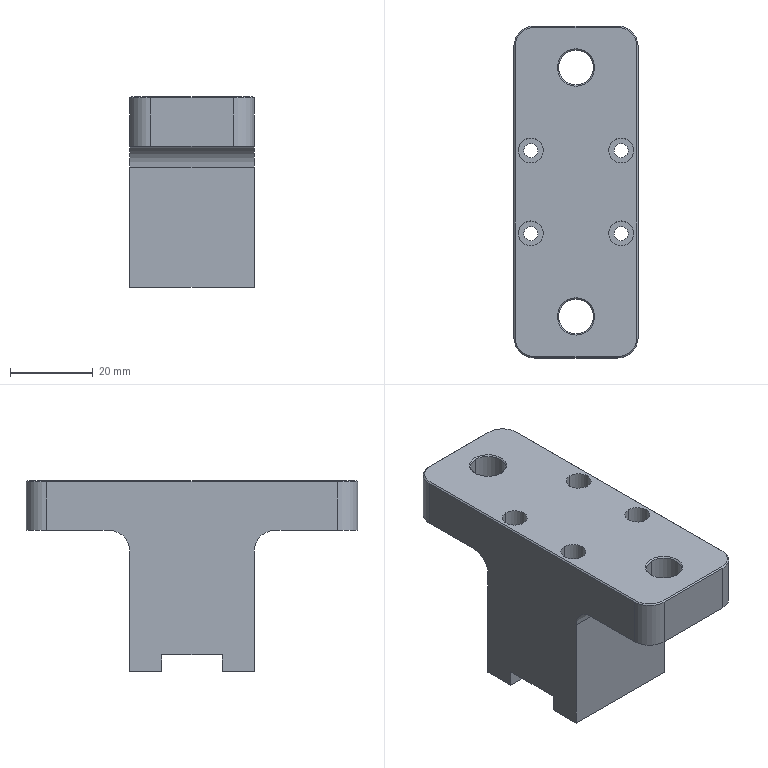NC program | NX | posted with a generic post | part box 30 x 80 x 46 mm
Lines 19 to 1040 of 3641:
(ZLEVEL_PROFILE , TOOL : D10)
N36 T15 M6
N38 G54
N40 G17 G0 G90 X-38.948 Y-19.275 S9500 M3
N42 G43 Z30. H15
N44 Z1.5
N46 G94 G1 X-39.694 Y-18.977 Z1.458 F1000.
N48 X-41.403 Y-17.85 Z1.351
N50 X-42.85 Y-16.403 Z1.243
N52 X-43.977 Y-14.694 Z1.136
N54 X-44.737 Y-12.793 Z1.029
N56 X-45.1 Y-10.779 Z0.922
N58 Y10.779 Z-0.208
N60 X-44.737 Y12.793 Z-0.316
N62 X-43.977 Y14.694 Z-0.423
N64 X-42.85 Y16.403 Z-0.53
N66 X-41.403 Y17.85 Z-0.637
N68 X-39.694 Y18.977 Z-0.745
N70 X-37.793 Y19.737 Z-0.852
N72 X-35.779 Y20.1 Z-0.959
N74 X-35. Z-1.
N76 X35. F3000.
N78 G2 X45.1 Y10. R10.1
N80 G1 Y-10.
N82 G2 X35. Y-20.1 R10.1
N84 G1 X-35.
N86 G2 X-45.1 Y-10. R10.1
N88 G1 Y10.
N90 G2 X-35. Y20.1 R10.1
N92 G1 X22.29 Z-2.
N94 X35.
N96 G2 X45.1 Y10. R10.1
N98 G1 Y-10.
N100 G2 X35. Y-20.1 R10.1
N102 G1 X-35.
N104 G2 X-45.1 Y-10. R10.1
N106 G1 Y10.
N108 G2 X-35. Y20.1 R10.1
N110 G1 X22.29 Z-3.
N112 X35.
N114 G2 X45.1 Y10. R10.1
N116 G1 Y-10.
N118 G2 X35. Y-20.1 R10.1
N120 G1 X-35.
N122 G2 X-45.1 Y-10. R10.1
N124 G1 Y10.
N126 G2 X-35. Y20.1 R10.1
N128 G1 X22.29 Z-4.
N130 X35.
N132 G2 X45.1 Y10. R10.1
N134 G1 Y-10.
N136 G2 X35. Y-20.1 R10.1
N138 G1 X-35.
N140 G2 X-45.1 Y-10. R10.1
N142 G1 Y10.
N144 G2 X-35. Y20.1 R10.1
N146 G1 X22.29 Z-5.
N148 X35.
N150 G2 X45.1 Y10. R10.1
N152 G1 Y-10.
N154 G2 X35. Y-20.1 R10.1
N156 G1 X-35.
N158 G2 X-45.1 Y-10. R10.1
N160 G1 Y10.
N162 G2 X-35. Y20.1 R10.1
N164 G1 X22.29 Z-6.
N166 X35.
N168 G2 X45.1 Y10. R10.1
N170 G1 Y-10.
N172 G2 X35. Y-20.1 R10.1
N174 G1 X-35.
N176 G2 X-45.1 Y-10. R10.1
N178 G1 Y10.
N180 G2 X-35. Y20.1 R10.1
N182 G1 X22.29 Z-7.
N184 X35.
N186 G2 X45.1 Y10. R10.1
N188 G1 Y-10.
N190 G2 X35. Y-20.1 R10.1
N192 G1 X-35.
N194 G2 X-45.1 Y-10. R10.1
N196 G1 Y10.
N198 G2 X-35. Y20.1 R10.1
N200 G1 X22.29 Z-8.
N202 X35.
N204 G2 X45.1 Y10. R10.1
N206 G1 Y-10.
N208 G2 X35. Y-20.1 R10.1
N210 G1 X-35.
N212 G2 X-45.1 Y-10. R10.1
N214 G1 Y10.
N216 G2 X-35. Y20.1 R10.1
N218 G1 X22.29 Z-9.
N220 X35.
N222 G2 X45.1 Y10. R10.1
N224 G1 Y-10.
N226 G2 X35. Y-20.1 R10.1
N228 G1 X-35.
N230 G2 X-45.1 Y-10. R10.1
N232 G1 Y10.
N234 G2 X-35. Y20.1 R10.1
N236 G1 X22.29 Z-10.
N238 X35.
N240 G2 X45.1 Y10. R10.1
N242 G1 Y-10.
N244 G2 X35. Y-20.1 R10.1
N246 G1 X-35.
N248 G2 X-45.1 Y-10. R10.1
N250 G1 Y10.
N252 G2 X-35. Y20.1 R10.1
N254 G1 X22.29 Z-11.
N256 X35.
N258 G2 X45.1 Y10. R10.1
N260 G1 Y-10.
N262 G2 X35. Y-20.1 R10.1
N264 G1 X-35.
N266 G2 X-45.1 Y-10. R10.1
N268 G1 Y10.
N270 G2 X-35. Y20.1 R10.1
N272 G1 X22.29 Z-12.
N274 X35.
N276 G2 X45.1 Y10. R10.1
N278 G1 Y-10.
N280 G2 X35. Y-20.1 R10.1
N282 G1 X-35.
N284 G2 X-45.1 Y-10. R10.1
N286 G1 Y10.
N288 G2 X-35. Y20.1 R10.1
N290 G1 X22.29 Z-13.
N292 X35.
N294 G2 X45.1 Y10. R10.1
N296 G1 Y-10.
N298 G2 X35. Y-20.1 R10.1
N300 G1 X-35.
N302 G2 X-45.1 Y-10. R10.1
N304 G1 Y10.
N306 G2 X-35. Y20.1 R10.1
N308 G1 X22.29 Z-14.
N310 X35.
N312 G2 X45.1 Y10. R10.1
N314 G1 Y-10.
N316 G2 X35. Y-20.1 R10.1
N318 G1 X-35.
N320 G2 X-45.1 Y-10. R10.1
N322 G1 Y10.
N324 G2 X-35. Y20.1 R10.1
N326 G1 X22.29 Z-15.
N328 X35.
N330 G2 X45.1 Y10. R10.1
N332 G1 Y-10.
N334 G2 X35. Y-20.1 R10.1
N336 G1 X-35.
N338 G2 X-45.1 Y-10. R10.1
N340 G1 Y10.
N342 G2 X-35. Y20.1 R10.1
N344 G1 X22.29 Z-16.
N346 X35.
N348 G2 X45.1 Y10. R10.1
N350 G1 Y-10.
N352 G2 X35. Y-20.1 R10.1
N354 G1 X-35.
N356 G2 X-45.1 Y-10. R10.1
N358 G1 Y10.
N360 G2 X-35. Y20.1 R10.1
N362 G1 X22.29 Z-17.
N364 X35.
N366 G2 X45.1 Y10. R10.1
N368 G1 Y-10.
N370 G2 X35. Y-20.1 R10.1
N372 G1 X-35.
N374 G2 X-45.1 Y-10. R10.1
N376 G1 Y10.
N378 G2 X-35. Y20.1 R10.1
N380 G1 X22.29 Z-18.
N382 X35.
N384 G2 X45.1 Y10. R10.1
N386 G1 Y-10.
N388 G2 X35. Y-20.1 R10.1
N390 G1 X-35.
N392 G2 X-45.1 Y-10. R10.1
N394 G1 Y10.
N396 G2 X-35. Y20.1 R10.1
N398 G1 X22.29 Z-19.
N400 X35.
N402 G2 X45.1 Y10. R10.1
N404 G1 Y-10.
N406 G2 X35. Y-20.1 R10.1
N408 G1 X-35.
N410 G2 X-45.1 Y-10. R10.1
N412 G1 Y10.
N414 G2 X-35. Y20.1 R10.1
N416 G1 X22.29 Z-20.
N418 X35.
N420 G2 X45.1 Y10. R10.1
N422 G1 Y-10.
N424 G2 X35. Y-20.1 R10.1
N426 G1 X-35.
N428 G2 X-45.1 Y-10. R10.1
N430 G1 Y10.
N432 G2 X-35. Y20.1 R10.1
N434 G1 X22.29 Z-21.
N436 X35.
N438 G2 X45.1 Y10. R10.1
N440 G1 Y-10.
N442 G2 X35. Y-20.1 R10.1
N444 G1 X-35.
N446 G2 X-45.1 Y-10. R10.1
N448 G1 Y10.
N450 G2 X-35. Y20.1 R10.1
N452 G1 X22.29 Z-22.
N454 X35.
N456 G2 X45.1 Y10. R10.1
N458 G1 Y-10.
N460 G2 X35. Y-20.1 R10.1
N462 G1 X-35.
N464 G2 X-45.1 Y-10. R10.1
N466 G1 Y10.
N468 G2 X-35. Y20.1 R10.1
N470 G1 X22.29 Z-23.
N472 X35.
N474 G2 X45.1 Y10. R10.1
N476 G1 Y-10.
N478 G2 X35. Y-20.1 R10.1
N480 G1 X-35.
N482 G2 X-45.1 Y-10. R10.1
N484 G1 Y10.
N486 G2 X-35. Y20.1 R10.1
N488 G1 X22.29 Z-24.
N490 X35.
N492 G2 X45.1 Y10. R10.1
N494 G1 Y-10.
N496 G2 X35. Y-20.1 R10.1
N498 G1 X-35.
N500 G2 X-45.1 Y-10. R10.1
N502 G1 Y10.
N504 G2 X-35. Y20.1 R10.1
N506 G1 X22.29 Z-25.
N508 X35.
N510 G2 X45.1 Y10. R10.1
N512 G1 Y-10.
N514 G2 X35. Y-20.1 R10.1
N516 G1 X-35.
N518 G2 X-45.1 Y-10. R10.1
N520 G1 Y10.
N522 G2 X-35. Y20.1 R10.1
N524 G1 X22.29 Z-26.
N526 X35.
N528 G2 X45.1 Y10. R10.1
N530 G1 Y-10.
N532 G2 X35. Y-20.1 R10.1
N534 G1 X-35.
N536 G2 X-45.1 Y-10. R10.1
N538 G1 Y10.
N540 G2 X-35. Y20.1 R10.1
N542 G1 X22.29 Z-27.
N544 X35.
N546 G2 X45.1 Y10. R10.1
N548 G1 Y-10.
N550 G2 X35. Y-20.1 R10.1
N552 G1 X-35.
N554 G2 X-45.1 Y-10. R10.1
N556 G1 Y10.
N558 G2 X-35. Y20.1 R10.1
N560 G1 X22.29 Z-28.
N562 X35.
N564 G2 X45.1 Y10. R10.1
N566 G1 Y-10.
N568 G2 X35. Y-20.1 R10.1
N570 G1 X-35.
N572 G2 X-45.1 Y-10. R10.1
N574 G1 Y10.
N576 G2 X-35. Y20.1 R10.1
N578 G1 X22.29 Z-29.
N580 X35.
N582 G2 X45.1 Y10. R10.1
N584 G1 Y-10.
N586 G2 X35. Y-20.1 R10.1
N588 G1 X-35.
N590 G2 X-45.1 Y-10. R10.1
N592 G1 Y10.
N594 G2 X-35. Y20.1 R10.1
N596 G1 X22.29 Z-30.
N598 X35.
N600 G2 X45.1 Y10. R10.1
N602 G1 Y-10.
N604 G2 X35. Y-20.1 R10.1
N606 G1 X-35.
N608 G2 X-45.1 Y-10. R10.1
N610 G1 Y10.
N612 G2 X-35. Y20.1 R10.1
N614 G1 X22.29 Z-31.
N616 X35.
N618 G2 X45.1 Y10. R10.1
N620 G1 Y-10.
N622 G2 X35. Y-20.1 R10.1
N624 G1 X-35.
N626 G2 X-45.1 Y-10. R10.1
N628 G1 Y10.
N630 G2 X-35. Y20.1 R10.1
N632 G1 X22.29 Z-32.
N634 X35.
N636 G2 X45.1 Y10. R10.1
N638 G1 Y-10.
N640 G2 X35. Y-20.1 R10.1
N642 G1 X-35.
N644 G2 X-45.1 Y-10. R10.1
N646 G1 Y10.
N648 G2 X-35. Y20.1 R10.1
N650 G1 X22.29 Z-33.
N652 X35.
N654 G2 X45.1 Y10. R10.1
N656 G1 Y-10.
N658 G2 X35. Y-20.1 R10.1
N660 G1 X-35.
N662 G2 X-45.1 Y-10. R10.1
N664 G1 Y10.
N666 G2 X-35. Y20.1 R10.1
N668 G1 X22.29 Z-34.
N670 X35.
N672 G2 X45.1 Y10. R10.1
N674 G1 Y-10.
N676 G2 X35. Y-20.1 R10.1
N678 G1 X-35.
N680 G2 X-45.1 Y-10. R10.1
N682 G1 Y10.
N684 G2 X-35. Y20.1 R10.1
N686 G1 X22.29 Z-35.
N688 X35.
N690 G2 X45.1 Y10. R10.1
N692 G1 Y-10.
N694 G2 X35. Y-20.1 R10.1
N696 G1 X-35.
N698 G2 X-45.1 Y-10. R10.1
N700 G1 Y10.
N702 G2 X-35. Y20.1 R10.1
N704 G1 X22.29 Z-36.
N706 X35.
N708 G2 X45.1 Y10. R10.1
N710 G1 Y-10.
N712 G2 X35. Y-20.1 R10.1
N714 G1 X-35.
N716 G2 X-45.1 Y-10. R10.1
N718 G1 Y10.
N720 G2 X-35. Y20.1 R10.1
N722 G1 X22.29 Z-37.
N724 X35.
N726 G2 X45.1 Y10. R10.1
N728 G1 Y-10.
N730 G2 X35. Y-20.1 R10.1
N732 G1 X-35.
N734 G2 X-45.1 Y-10. R10.1
N736 G1 Y10.
N738 G2 X-35. Y20.1 R10.1
N740 G1 X22.29 Z-38.
N742 X35.
N744 G2 X45.1 Y10. R10.1
N746 G1 Y-10.
N748 G2 X35. Y-20.1 R10.1
N750 G1 X-35.
N752 G2 X-45.1 Y-10. R10.1
N754 G1 Y10.
N756 G2 X-35. Y20.1 R10.1
N758 G1 X22.29 Z-39.
N760 X35.
N762 G2 X45.1 Y10. R10.1
N764 G1 Y-10.
N766 G2 X35. Y-20.1 R10.1
N768 G1 X-35.
N770 G2 X-45.1 Y-10. R10.1
N772 G1 Y10.
N774 G2 X-35. Y20.1 R10.1
N776 G1 X22.29 Z-40.
N778 X35.
N780 G2 X45.1 Y10. R10.1
N782 G1 Y-10.
N784 G2 X35. Y-20.1 R10.1
N786 G1 X-35.
N788 G2 X-45.1 Y-10. R10.1
N790 G1 Y10.
N792 G2 X-35. Y20.1 R10.1
N794 G1 X22.29 Z-41.
N796 X35.
N798 G2 X45.1 Y10. R10.1
N800 G1 Y-10.
N802 G2 X35. Y-20.1 R10.1
N804 G1 X-35.
N806 G2 X-45.1 Y-10. R10.1
N808 G1 Y10.
N810 G2 X-35. Y20.1 R10.1
N812 G1 X22.29 Z-42.
N814 X35.
N816 G2 X45.1 Y10. R10.1
N818 G1 Y-10.
N820 G2 X35. Y-20.1 R10.1
N822 G1 X-35.
N824 G2 X-45.1 Y-10. R10.1
N826 G1 Y10.
N828 G2 X-35. Y20.1 R10.1
N830 G1 X22.29 Z-43.
N832 X35.
N834 G2 X45.1 Y10. R10.1
N836 G1 Y-10.
N838 G2 X35. Y-20.1 R10.1
N840 G1 X-35.
N842 G2 X-45.1 Y-10. R10.1
N844 G1 Y10.
N846 G2 X-35. Y20.1 R10.1
N848 G1 X22.29 Z-44.
N850 X35.
N852 G2 X45.1 Y10. R10.1
N854 G1 Y-10.
N856 G2 X35. Y-20.1 R10.1
N858 G1 X-35.
N860 G2 X-45.1 Y-10. R10.1
N862 G1 Y10.
N864 G2 X-35. Y20.1 R10.1
N866 G1 X22.29 Z-45.
N868 X35.
N870 G2 X45.1 Y10. R10.1
N872 G1 Y-10.
N874 G2 X35. Y-20.1 R10.1
N876 G1 X-35.
N878 G2 X-45.1 Y-10. R10.1
N880 G1 Y10.
N882 G2 X-35. Y20.1 R10.1
N884 G1 X22.29 Z-46.
N886 X35.
N888 G2 X45.1 Y10. R10.1
N890 G1 Y-10.
N892 G2 X35. Y-20.1 R10.1
N894 G1 X-35.
N896 G2 X-45.1 Y-10. R10.1
N898 G1 Y10.
N900 G2 X-35. Y20.1 R10.1
N902 G1 X22.29
N904 Z-44.5
N906 G0 Z30.
(ZLEVEL_PROFILE_COPY_COPY_COPY , TOOL : D10)
N908 X40.999 Y21.367
N910 Z-0.997
N912 G1 X39.499 Y20.501 F1000.
N914 G3 X38.999 Y19.635 R1.
N916 G1 X39. Y14.376 F3000.
N918 Y-15.
N920 X38.999 Y-19.635
N922 G3 X39.499 Y-20.501 R1.
N924 G1 X40.999 Y-21.367
N926 G0 X40.998 Y-21.395 Z-1.994
N928 G1 X39.499 Y-20.529 F1000.
N930 G2 X38.999 Y-19.663 R1.
N932 G1 X39. Y-15. F3000.
N934 Y14.376
N936 X38.999 Y19.663
N938 G2 X39.499 Y20.529 R1.
N940 G1 X40.998 Y21.395
N942 G0 X40.996 Y21.422 Z-2.991
N944 G1 X39.499 Y20.558 F1000.
N946 G3 X38.999 Y19.692 R1.
N948 G1 X39. Y14.376 F3000.
N950 Y-15.
N952 X38.999 Y-19.692
N954 G3 X39.499 Y-20.558 R1.
N956 G1 X40.996 Y-21.422
N958 G0 X40.994 Y-21.449 Z-3.988
N960 G1 X39.499 Y-20.586 F1000.
N962 G2 X38.999 Y-19.72 R1.
N964 G1 X39. Y-15. F3000.
N966 Y14.376
N968 X38.999 Y19.72
N970 G2 X39.499 Y20.586 R1.
N972 G1 X40.994 Y21.449
N974 G0 X40.992 Y21.477 Z-4.985
N976 G1 X39.499 Y20.615 F1000.
N978 G3 X38.999 Y19.749 R1.
N980 G1 X39. Y14.376 F3000.
N982 Y-15.
N984 X38.999 Y-19.748
N986 G3 X39.499 Y-20.615 R1.
N988 G1 X40.992 Y-21.477
N990 G0 X40.99 Y-21.504 Z-5.982
N992 G1 X39.499 Y-20.643 F1000.
N994 G2 X38.999 Y-19.777 R1.
N996 G1 X39. Y-15. F3000.
N998 Y14.376
N1000 X38.999 Y19.777
N1002 G2 X39.499 Y20.643 R1.
N1004 G1 X40.99 Y21.504
N1006 G0 X40.988 Y21.548 Z-6.979
N1008 G1 X39.494 Y20.674 F1000.
N1010 G3 X38.999 Y19.805 R1.
N1012 G1 X39.001 Y19.45 F3000.
N1014 X39. Y14.376
N1016 Y-15.
N1018 X39.001 Y-19.45
N1020 X38.999 Y-19.805
N1022 G3 X39.494 Y-20.674 R1.
N1024 G1 X40.988 Y-21.548
N1026 G0 X40.986 Y-21.575 Z-7.976
N1028 G1 X39.494 Y-20.702 F1000.
N1030 G2 X38.999 Y-19.834 R1.
N1032 G1 X39.002 Y-19.45 F3000.
N1034 X39. Y-15.
N1036 Y14.376
N1038 X39.002 Y19.45
N1040 X38.999 Y19.834
N1042 G2 X39.494 Y20.703 R1.
N1044 G1 X40.986 Y21.575
N1046 G0 X40.984 Y21.603 Z-8.974
N1048 G1 X39.494 Y20.731 F1000.
N1050 G3 X38.999 Y19.862 R1.
N1052 G1 X39.002 Y19.45 F3000.
N1054 X39. Y14.376
N1056 Y-15.
N1058 X39.002 Y-19.45
N1060 X38.999 Y-19.862
N1062 G3 X39.494 Y-20.731 R1.
N1064 G1 X40.984 Y-21.603
N1066 G0 X40.982 Y-21.63 Z-9.971
N1068 G1 X39.494 Y-20.759 F1000.
N1070 G2 X38.999 Y-19.89 R1.
N1072 G1 X39.002 Y-19.45 F3000.
N1074 X39. Y-15.
N1076 Y14.376
N1078 X39.002 Y19.45
N1080 X38.999 Y19.89
N1082 G2 X39.494 Y20.759 R1.
N1084 G1 X40.982 Y21.63
N1086 G0 X40.98 Y21.658 Z-10.968
N1088 G1 X39.494 Y20.788 F1000.
N1090 G3 X38.999 Y19.919 R1.
N1092 G1 X39.002 Y19.45 F3000.
N1094 X39. Y14.376
N1096 Y-15.
N1098 X39.002 Y-19.45
N1100 X38.999 Y-19.919
N1102 G3 X39.494 Y-20.788 R1.
N1104 G1 X40.98 Y-21.658
N1106 G0 X40.978 Y-21.685 Z-11.965
N1108 G1 X39.494 Y-20.816 F1000.
N1110 G2 X38.999 Y-19.947 R1.
N1112 G1 X39.002 Y-19.45 F3000.
N1114 X39. Y-15.
N1116 Y14.376
N1118 X39.002 Y19.45
N1120 X38.999 Y19.947
N1122 G2 X39.494 Y20.816 R1.
N1124 G1 X40.978 Y21.685
N1126 G0 X40.976 Y21.713 Z-12.962
N1128 G1 X39.494 Y20.844 F1000.
N1130 G3 X38.999 Y19.975 R1.
N1132 G1 X39.002 Y19.45 F3000.
N1134 X39. Y14.376
N1136 Y-15.
N1138 X39.002 Y-19.45
N1140 X38.999 Y-19.975
N1142 G3 X39.494 Y-20.844 R1.
N1144 G1 X40.976 Y-21.713
N1146 G0 X40.974 Y-21.74 Z-13.959
N1148 G1 X39.493 Y-20.873 F1000.
N1150 G2 X38.999 Y-20.004 R1.
N1152 G1 X39.002 Y-19.45 F3000.
N1154 X39. Y-15.
N1156 Y14.376
N1158 X39.002 Y19.45
N1160 X38.999 Y20.004
N1162 G2 X39.493 Y20.873 R1.
N1164 G1 X40.974 Y21.74
N1166 G0 X40.972 Y21.768 Z-14.956
N1168 G1 X39.493 Y20.901 F1000.
N1170 G3 X38.999 Y20.032 R1.
N1172 G1 X39.003 Y19.45 F3000.
N1174 X39. Y14.376
N1176 Y-15.
N1178 X39.003 Y-19.45
N1180 X38.999 Y-20.032
N1182 G3 X39.493 Y-20.901 R1.
N1184 G1 X40.972 Y-21.768
N1186 G0 X40.97 Y-21.795 Z-15.953
N1188 G1 X39.493 Y-20.93 F1000.
N1190 G2 X38.999 Y-20.06 R1.
N1192 G1 X39.003 Y-19.45 F3000.
N1194 X39. Y-15.
N1196 Y14.376
N1198 X39.003 Y19.45
N1200 X38.999 Y20.06
N1202 G2 X39.493 Y20.93 R1.
N1204 G1 X40.97 Y21.795
N1206 G0 X40.968 Y21.823 Z-16.95
N1208 G1 X39.493 Y20.958 F1000.
N1210 G3 X38.999 Y20.089 R1.
N1212 G1 X39.003 Y19.45 F3000.
N1214 X39. Y14.376
N1216 Y-15.
N1218 X39.003 Y-19.45
N1220 X38.999 Y-20.089
N1222 G3 X39.493 Y-20.958 R1.
N1224 G1 X40.968 Y-21.823
N1226 G0 X40.967 Y-21.85 Z-17.947
N1228 G1 X39.493 Y-20.986 F1000.
N1230 G2 X38.999 Y-20.117 R1.
N1232 G1 X39.003 Y-19.45 F3000.
N1234 X39. Y-15.
N1236 Y14.376
N1238 X39.003 Y19.45
N1240 X38.999 Y20.117
N1242 G2 X39.493 Y20.986 R1.
N1244 G1 X40.967 Y21.85
N1246 G0 X40.965 Y21.878 Z-18.944
N1248 G1 X39.493 Y21.015 F1000.
N1250 G3 X38.998 Y20.145 R1.
N1252 G1 X39.003 Y19.45 F3000.
N1254 X39. Y14.376
N1256 Y-15.
N1258 X39.003 Y-19.45
N1260 X38.998 Y-20.145
N1262 G3 X39.493 Y-21.015 R1.
N1264 G1 X40.965 Y-21.878
N1266 G0 X40.963 Y-21.905 Z-19.941
N1268 G1 X39.493 Y-21.043 F1000.
N1270 G2 X38.998 Y-20.174 R1.
N1272 G1 X39.003 Y-19.45 F3000.
N1274 X39. Y-15.
N1276 Y14.376
N1278 Y15.021
N1280 X39.003 Y19.45
N1282 X38.998 Y20.174
N1284 G2 X39.493 Y21.043 R1.
N1286 G1 X40.963 Y21.905
N1288 G0 X40.961 Y21.933 Z-20.938
N1290 G1 X39.492 Y21.071 F1000.
N1292 G3 X38.998 Y20.202 R1.
N1294 G1 X39.003 Y19.45 F3000.
N1296 X39. Y15.021
N1298 Y14.376
N1300 Y-15.
N1302 X39.003 Y-19.45
N1304 X38.998 Y-20.202
N1306 G3 X39.492 Y-21.071 R1.
N1308 G1 X40.961 Y-21.933
N1310 G0 X40.959 Y-21.96 Z-21.935
N1312 G1 X39.492 Y-21.1 F1000.
N1314 G2 X38.998 Y-20.23 R1.
N1316 G1 X39.004 Y-19.45 F3000.
N1318 X39. Y-15.
N1320 Y14.376
N1322 Y15.021
N1324 X39.004 Y19.45
N1326 X38.998 Y20.23
N1328 G2 X39.492 Y21.1 R1.
N1330 G1 X40.959 Y21.96
N1332 G0 X40.957 Y21.988 Z-22.932
N1334 G1 X39.492 Y21.128 F1000.
N1336 G3 X38.998 Y20.259 R1.
N1338 G1 X39.004 Y19.45 F3000.
N1340 X39. Y15.021
N1342 Y14.376
N1344 Y-15.
N1346 X39.004 Y-19.45
N1348 X38.998 Y-20.259
N1350 G3 X39.492 Y-21.128 R1.
N1352 G1 X40.957 Y-21.987
N1354 G0 X40.955 Y-22.015 Z-23.929
N1356 G1 X39.492 Y-21.156 F1000.
N1358 G2 X38.998 Y-20.287 R1.
N1360 G1 X39.004 Y-19.45 F3000.
N1362 X39. Y-15.
N1364 Y14.376
N1366 Y15.021
N1368 X39.004 Y19.45
N1370 X38.998 Y20.287
N1372 G2 X39.492 Y21.157 R1.
N1374 G1 X40.955 Y22.015
N1376 G0 X40.954 Y22.023 Z-24.926
N1378 G1 X39.498 Y21.182 F1000.
N1380 G3 X38.998 Y20.315 R1.
N1382 G1 X39. Y14.376 F3000.
N1384 Y-15.
N1386 X39.004 Y-19.45
N1388 X38.998 Y-20.315
N1390 G3 X39.492 Y-21.185 R1.
N1392 G1 X40.953 Y-22.042
N1394 G0 X40.951 Y-22.07 Z-25.924
N1396 G1 X39.491 Y-21.213 F1000.
N1398 G2 X38.998 Y-20.343 R1.
N1400 G1 X39.004 Y-19.45 F3000.
N1402 X39. Y-15.
N1404 Y14.376
N1406 X38.998 Y20.344
N1408 G2 X39.497 Y21.21 R1.
N1410 G1 X40.952 Y22.051
N1412 G0 X40.95 Y22.078 Z-26.921
N1414 G1 X39.497 Y21.238 F1000.
N1416 G3 X38.998 Y20.372 R1.
N1418 G1 X39. Y14.376 F3000.
N1420 Y-15.
N1422 X39.004 Y-19.45
N1424 X38.998 Y-20.372
N1426 G3 X39.491 Y-21.241 R1.
N1428 G1 X40.949 Y-22.097
N1430 G0 X40.947 Y-22.125 Z-27.918
N1432 G1 X39.491 Y-21.27 F1000.
N1434 G2 X38.997 Y-20.4 R1.
N1436 G1 X39.004 Y-19.45 F3000.
N1438 X39. Y-15.
N1440 Y14.376
N1442 X38.997 Y20.4
N1444 G2 X39.497 Y21.266 R1.
N1446 G1 X40.948 Y22.105
N1448 G0 X40.946 Y22.132 Z-28.915
N1450 G1 X39.497 Y21.295 F1000.
N1452 G3 X38.997 Y20.429 R1.
N1454 G1 X38.999 Y14.793 F3000.
N1456 X39. Y14.376
N1458 Y-15.
N1460 X39.005 Y-19.45
N1462 X38.997 Y-20.428
N1464 G3 X39.491 Y-21.298 R1.
N1466 G1 X40.945 Y-22.152
N1468 G0 X41.131 Y-22.176 Z-29.912
N1470 G1 X39.68 Y-21.33 F1000.
N1472 G2 X39.184 Y-20.462 R1.
N1474 G3 X39.084 Y-14.689 R134.164 F3000.
N1476 G1 Y14.793
N1478 G3 X39.165 Y20.459 R86.418
N1480 G2 X39.649 Y21.334 R1.
N1482 G1 X41.109 Y22.214
N1484 G0 X41.473 Y22.246 Z-30.909
N1486 G1 X39.998 Y21.363 F1000.
N1488 G3 X39.512 Y20.49 R1.
N1490 G2 X39.435 Y14.974 R93.208 F3000.
N1492 G1 X39.411 Y14.61
N1494 X39.379 Y14.552
N1496 Y-14.534
N1498 X39.405 Y-14.614
N1500 X39.49 Y-16.067
N1502 X39.499 Y-16.7
N1504 X39.512 Y-20.489
N1506 G3 X40.015 Y-21.354 R1.
N1508 G1 X41.463 Y-22.183
N1510 G0 X42.044 Y-22.251 Z-31.906
N1512 G1 X40.585 Y-21.374 F1000.
N1514 G2 X40.101 Y-20.499 R1.
N1516 G3 X39.975 Y-14.376 R79.288 F3000.
N1518 G1 X39.931 Y-14.264
N1520 Y14.264
N1522 X39.975 Y14.376
N1524 G3 X40.101 Y20.499 R79.291
N1526 G2 X40.585 Y21.374 R1.
N1528 G1 X42.044 Y22.252
N1530 G0 X43.052 Y22.297 Z-32.903
N1532 G1 X41.589 Y21.382 F1000.
N1534 G3 X41.12 Y20.5 R1.
N1536 G2 X40.875 Y13.953 R45.316 F3000.
N1538 G1 Y-13.953
N1540 G2 X41.12 Y-20.499 R45.314
N1542 G3 X41.589 Y-21.382 R1.
N1544 G1 X43.059 Y-22.301
N1546 G0 X45.387 Y-21.571 Z-33.9
N1548 G1 X43.95 Y-20.813 F1000.
N1550 G2 X43.417 Y-19.966 R1.
N1552 G1 X43.205 Y-14.376 F3000.
N1554 X43.005 Y-13.22
N1556 Y13.869
N1558 X43.136 Y14.376
N1560 X43.468 Y19.894
N1562 G2 X44.019 Y20.729 R1.
N1564 G1 X45.359 Y21.399
N1566 G0 Z30.
N1568 X-40.999 Y-21.367
N1570 Z-0.997
N1572 G1 X-39.499 Y-20.501 F1000.
N1574 G3 X-38.999 Y-19.635 R1.
N1576 G1 X-39. Y-14.961 F3000.
N1578 Y14.376
N1580 X-38.999 Y19.635
N1582 G3 X-39.499 Y20.501 R1.
N1584 G1 X-40.999 Y21.367
N1586 G0 X-40.998 Y21.395 Z-1.994
N1588 G1 X-39.499 Y20.529 F1000.
N1590 G2 X-38.999 Y19.663 R1.
N1592 G1 X-39. Y14.376 F3000.
N1594 Y-14.961
N1596 X-38.999 Y-19.663
N1598 G2 X-39.499 Y-20.529 R1.
N1600 G1 X-40.998 Y-21.395
N1602 G0 X-40.996 Y-21.422 Z-2.991
N1604 G1 X-39.499 Y-20.558 F1000.
N1606 G3 X-38.999 Y-19.692 R1.
N1608 G1 X-39. Y-14.961 F3000.
N1610 Y14.376
N1612 X-38.999 Y19.692
N1614 G3 X-39.499 Y20.558 R1.
N1616 G1 X-40.996 Y21.422
N1618 G0 X-40.994 Y21.449 Z-3.988
N1620 G1 X-39.499 Y20.586 F1000.
N1622 G2 X-38.999 Y19.72 R1.
N1624 G1 X-39. Y14.376 F3000.
N1626 Y-14.961
N1628 X-38.999 Y-19.72
N1630 G2 X-39.499 Y-20.586 R1.
N1632 G1 X-40.994 Y-21.449
N1634 G0 X-40.992 Y-21.477 Z-4.985
N1636 G1 X-39.499 Y-20.615 F1000.
N1638 G3 X-38.999 Y-19.748 R1.
N1640 G1 X-39. Y-14.961 F3000.
N1642 Y14.376
N1644 X-38.999 Y19.749
N1646 G3 X-39.499 Y20.615 R1.
N1648 G1 X-40.992 Y21.477
N1650 G0 X-40.99 Y21.504 Z-5.982
N1652 G1 X-39.499 Y20.643 F1000.
N1654 G2 X-38.999 Y19.777 R1.
N1656 G1 X-39. Y14.376 F3000.
N1658 Y-14.961
N1660 X-38.999 Y-19.777
N1662 G2 X-39.499 Y-20.643 R1.
N1664 G1 X-40.99 Y-21.504
N1666 G0 X-40.988 Y-21.548 Z-6.979
N1668 G1 X-39.494 Y-20.674 F1000.
N1670 G3 X-38.999 Y-19.805 R1.
N1672 G1 X-39.001 Y-19.45 F3000.
N1674 X-39. Y-14.961
N1676 Y14.376
N1678 X-39.001 Y19.45
N1680 X-38.999 Y19.805
N1682 G3 X-39.494 Y20.674 R1.
N1684 G1 X-40.988 Y21.548
N1686 G0 X-40.986 Y21.575 Z-7.976
N1688 G1 X-39.494 Y20.703 F1000.
N1690 G2 X-38.999 Y19.834 R1.
N1692 G1 X-39.002 Y19.45 F3000.
N1694 X-39. Y14.376
N1696 Y-14.961
N1698 X-39.002 Y-19.45
N1700 X-38.999 Y-19.834
N1702 G2 X-39.494 Y-20.702 R1.
N1704 G1 X-40.986 Y-21.575
N1706 G0 X-40.984 Y-21.603 Z-8.974
N1708 G1 X-39.494 Y-20.731 F1000.
N1710 G3 X-38.999 Y-19.862 R1.
N1712 G1 X-39.002 Y-19.45 F3000.
N1714 X-39. Y-14.961
N1716 Y14.376
N1718 X-39.002 Y19.45
N1720 X-38.999 Y19.862
N1722 G3 X-39.494 Y20.731 R1.
N1724 G1 X-40.984 Y21.603
N1726 G0 X-40.982 Y21.63 Z-9.971
N1728 G1 X-39.494 Y20.759 F1000.
N1730 G2 X-38.999 Y19.89 R1.
N1732 G1 X-39.002 Y19.45 F3000.
N1734 X-39. Y14.376
N1736 Y-14.961
N1738 X-38.999 Y-19.89
N1740 G2 X-39.499 Y-20.756 R1.
N1742 G1 X-40.983 Y-21.613
N1744 G0 X-40.981 Y-21.641 Z-10.968
N1746 G1 X-39.499 Y-20.785 F1000.
N1748 G3 X-38.999 Y-19.919 R1.
N1750 G1 X-39. Y-14.961 F3000.
N1752 Y14.376
N1754 X-39.002 Y19.45
N1756 X-38.999 Y19.919
N1758 G3 X-39.494 Y20.788 R1.
N1760 G1 X-40.98 Y21.658
N1762 G0 X-40.978 Y21.685 Z-11.965
N1764 G1 X-39.494 Y20.816 F1000.
N1766 G2 X-38.999 Y19.947 R1.
N1768 G1 X-39.002 Y19.45 F3000.
N1770 X-39. Y14.376
N1772 Y-14.961
N1774 X-38.999 Y-19.947
N1776 G2 X-39.499 Y-20.813 R1.
N1778 G1 X-40.979 Y-21.668
N1780 G0 X-40.977 Y-21.695 Z-12.962
N1782 G1 X-39.499 Y-20.841 F1000.
N1784 G3 X-38.999 Y-19.975 R1.
N1786 G1 X-39. Y-14.961 F3000.
N1788 Y14.376
N1790 X-39.002 Y19.45
N1792 X-38.999 Y19.975
N1794 G3 X-39.494 Y20.844 R1.
N1796 G1 X-40.976 Y21.713
N1798 G0 X-40.974 Y21.74 Z-13.959
N1800 G1 X-39.493 Y20.873 F1000.
N1802 G2 X-38.999 Y20.004 R1.
N1804 G1 X-39.002 Y19.45 F3000.
N1806 X-39. Y14.376
N1808 Y-14.961
N1810 X-38.999 Y-20.004
N1812 G2 X-39.499 Y-20.87 R1.
N1814 G1 X-40.975 Y-21.723
N1816 G0 X-40.973 Y-21.75 Z-14.956
N1818 G1 X-39.499 Y-20.898 F1000.
N1820 G3 X-38.999 Y-20.032 R1.
N1822 G1 X-39. Y-14.961 F3000.
N1824 Y14.376
N1826 X-39.003 Y19.45
N1828 X-38.999 Y20.032
N1830 G3 X-39.493 Y20.901 R1.
N1832 G1 X-40.972 Y21.768
N1834 G0 X-40.97 Y21.795 Z-15.953
N1836 G1 X-39.493 Y20.93 F1000.
N1838 G2 X-38.999 Y20.06 R1.
N1840 G1 X-39.003 Y19.45 F3000.
N1842 X-39. Y14.376
N1844 Y-14.961
N1846 X-39.003 Y-19.45
N1848 X-38.999 Y-20.06
N1850 G2 X-39.493 Y-20.93 R1.
N1852 G1 X-40.97 Y-21.795
N1854 G0 X-40.968 Y-21.823 Z-16.95
N1856 G1 X-39.493 Y-20.958 F1000.
N1858 G3 X-38.999 Y-20.089 R1.
N1860 G1 X-39.003 Y-19.45 F3000.
N1862 X-39. Y-14.961
N1864 Y14.376
N1866 X-39.003 Y19.45
N1868 X-38.999 Y20.089
N1870 G3 X-39.493 Y20.958 R1.
N1872 G1 X-40.968 Y21.823
N1874 G0 X-40.967 Y21.85 Z-17.947
N1876 G1 X-39.493 Y20.986 F1000.
N1878 G2 X-38.999 Y20.117 R1.
N1880 G1 X-39.003 Y19.45 F3000.
N1882 X-39. Y14.376
N1884 Y-14.961
N1886 X-39.003 Y-19.45
N1888 X-38.999 Y-20.117
N1890 G2 X-39.493 Y-20.986 R1.
N1892 G1 X-40.967 Y-21.85
N1894 G0 X-40.965 Y-21.878 Z-18.944
N1896 G1 X-39.493 Y-21.015 F1000.
N1898 G3 X-38.998 Y-20.145 R1.
N1900 G1 X-39.003 Y-19.45 F3000.
N1902 X-39. Y-14.961
N1904 Y14.376
N1906 X-39.003 Y19.45
N1908 X-38.998 Y20.145
N1910 G3 X-39.493 Y21.015 R1.
N1912 G1 X-40.965 Y21.878
N1914 G0 X-40.963 Y21.905 Z-19.941
N1916 G1 X-39.493 Y21.043 F1000.
N1918 G2 X-38.998 Y20.174 R1.
N1920 G1 X-39.003 Y19.45 F3000.
N1922 X-39. Y14.376
N1924 Y-14.961
N1926 X-39.003 Y-19.45
N1928 X-38.998 Y-20.174
N1930 G2 X-39.493 Y-21.043 R1.
N1932 G1 X-40.963 Y-21.905
N1934 G0 X-40.961 Y-21.933 Z-20.938
N1936 G1 X-39.492 Y-21.071 F1000.
N1938 G3 X-38.998 Y-20.202 R1.
N1940 G1 X-39.003 Y-19.45 F3000.
N1942 X-39. Y-14.961
N1944 Y14.376
N1946 X-39.003 Y19.45
N1948 X-38.998 Y20.202
N1950 G3 X-39.492 Y21.071 R1.
N1952 G1 X-40.961 Y21.933
N1954 G0 X-40.959 Y21.96 Z-21.935
N1956 G1 X-39.492 Y21.1 F1000.
N1958 G2 X-38.998 Y20.23 R1.
N1960 G1 X-39.004 Y19.45 F3000.
N1962 X-39. Y14.376
N1964 Y-14.961
N1966 X-39.004 Y-19.45
N1968 X-38.998 Y-20.23
N1970 G2 X-39.492 Y-21.1 R1.
N1972 G1 X-40.959 Y-21.96
N1974 G0 X-40.957 Y-21.987 Z-22.932
N1976 G1 X-39.492 Y-21.128 F1000.
N1978 G3 X-38.998 Y-20.259 R1.
N1980 G1 X-39.004 Y-19.45 F3000.
N1982 X-39. Y-14.961
N1984 Y14.376
N1986 X-39.004 Y19.45
N1988 X-38.998 Y20.259
N1990 G3 X-39.492 Y21.128 R1.
N1992 G1 X-40.957 Y21.988
N1994 G0 X-40.955 Y22.015 Z-23.929
N1996 G1 X-39.492 Y21.157 F1000.
N1998 G2 X-38.998 Y20.287 R1.
N2000 G1 X-39.004 Y19.45 F3000.
N2002 X-39. Y14.376
N2004 Y-14.961
N2006 X-38.998 Y-20.287
N2008 G2 X-39.498 Y-21.153 R1.
N2010 G1 X-40.956 Y-21.996
N2012 G0 X-40.954 Y-22.023 Z-24.926
N2014 G1 X-39.497 Y-21.181 F1000.
N2016 G3 X-38.998 Y-20.315 R1.
N2018 G1 X-39. Y-14.961 F3000.
N2020 Y14.376
N2022 X-39.004 Y19.45
N2024 X-38.998 Y20.315
N2026 G3 X-39.492 Y21.185 R1.
N2028 G1 X-40.953 Y22.043
N2030 G0 X-40.951 Y22.07 Z-25.924
N2032 G1 X-39.491 Y21.213 F1000.
N2034 G2 X-38.998 Y20.344 R1.
N2036 G1 X-39.004 Y19.45 F3000.
N2038 X-39. Y14.376
N2040 Y-14.961
N2042 X-38.998 Y-20.343
N2044 G2 X-39.497 Y-21.21 R1.
N2046 G1 X-40.952 Y-22.05
N2048 G0 X-40.95 Y-22.078 Z-26.921
N2050 G1 X-39.497 Y-21.238 F1000.
N2052 G3 X-38.998 Y-20.372 R1.
N2054 G1 X-39. Y-14.961 F3000.
N2056 Y14.376
N2058 X-39.004 Y19.45
N2060 X-38.998 Y20.372
N2062 G3 X-39.491 Y21.242 R1.
N2064 G1 X-40.949 Y22.097
N2066 G0 X-40.947 Y22.125 Z-27.918